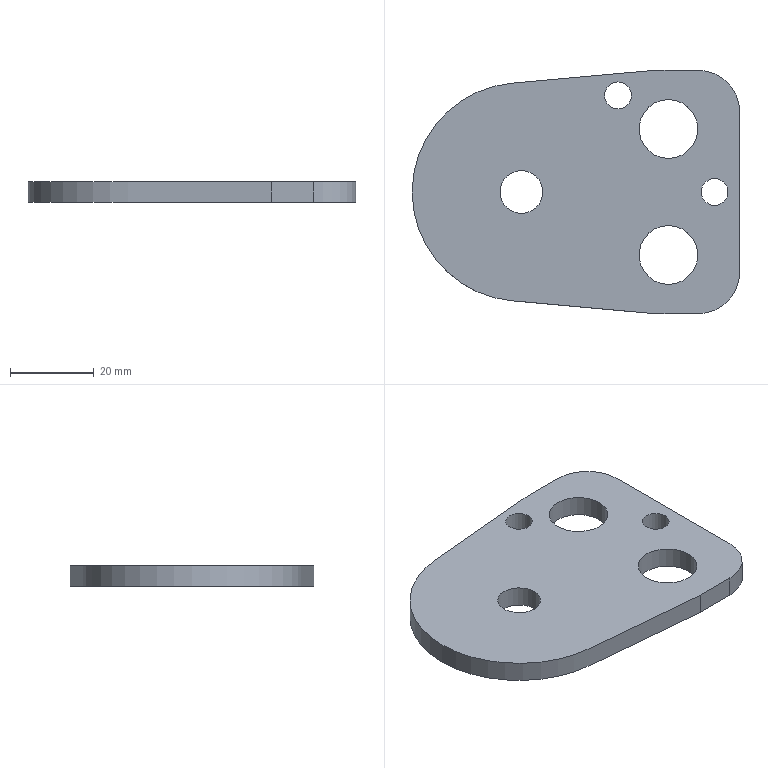Part | NX | features solid 2 | 1 solid | 17 faces | box 78 x 58 x 5 mm | volume 17443 mm3 | plane 9 | cylinder 8 | commonest cylinder face diameters 6.4 x2 14 x2 20 x2 10.2 x1 52 x1
STEP:
#1=CARTESIAN_POINT('',(-809.43,-240.038,136.));
#2=VERTEX_POINT('',#1);
#3=CARTESIAN_POINT('',(-809.43,-240.038,131.));
#4=VERTEX_POINT('',#3);
#5=CARTESIAN_POINT('',(-809.43,-240.038,131.));
#6=DIRECTION('',(0.,0.,-1.));
#7=VECTOR('',#6,1000.);
#8=LINE('',#5,#7);
#9=EDGE_CURVE('',#2,#4,#8,.T.);
#10=ORIENTED_EDGE('',*,*,#9,.F.);
#11=CARTESIAN_POINT('',(-809.43,-240.038,136.));
#12=VERTEX_POINT('',#11);
#13=CARTESIAN_POINT('',(-809.43,-214.144,136.));
#14=DIRECTION('',(0.,1.,0.));
#15=VECTOR('',#14,1000.);
#16=LINE('',#13,#15);
#17=EDGE_CURVE('',#2,#12,#16,.T.);
#18=ORIENTED_EDGE('',*,*,#17,.T.);
#19=CARTESIAN_POINT('',(-809.43,-240.038,131.));
#20=VERTEX_POINT('',#19);
#21=CARTESIAN_POINT('',(-809.43,-240.038,131.));
#22=DIRECTION('',(0.,0.,1.));
#23=VECTOR('',#22,1000.);
#24=LINE('',#21,#23);
#25=EDGE_CURVE('',#20,#12,#24,.T.);
#26=ORIENTED_EDGE('',*,*,#25,.F.);
#27=CARTESIAN_POINT('',(-809.43,-214.144,131.));
#28=DIRECTION('',(0.,-1.,0.));
#29=VECTOR('',#28,1000.);
#30=LINE('',#27,#29);
#31=EDGE_CURVE('',#20,#4,#30,.T.);
#32=ORIENTED_EDGE('',*,*,#31,.T.);
#33=EDGE_LOOP('',(#10,#18,#26,#32));
#34=FACE_BOUND('',#33,.T.);
#35=CARTESIAN_POINT('',(-809.43,-214.144,131.));
#36=DIRECTION('',(-1.,0.,0.));
#37=DIRECTION('',(0.,0.,1.));
#38=AXIS2_PLACEMENT_3D('',#35,#36,#37);
#39=PLANE('',#38);
#40=ADVANCED_FACE('',(#34),#39,.T.);
#41=CARTESIAN_POINT('',(-775.09,-185.144,136.));
#42=VERTEX_POINT('',#41);
#43=CARTESIAN_POINT('',(-809.43,-188.249,136.));
#44=VERTEX_POINT('',#43);
#45=CARTESIAN_POINT('',(-795.009,-186.945,136.));
#46=DIRECTION('',(-0.9959,-0.09007,0.));
#47=VECTOR('',#46,1000.);
#48=LINE('',#45,#47);
#49=EDGE_CURVE('',#42,#44,#48,.T.);
#50=ORIENTED_EDGE('',*,*,#49,.T.);
#51=CARTESIAN_POINT('',(-809.43,-188.249,136.));
#52=VERTEX_POINT('',#51);
#53=CARTESIAN_POINT('',(-809.43,-214.144,136.));
#54=DIRECTION('',(0.,1.,0.));
#55=VECTOR('',#54,1000.);
#56=LINE('',#53,#55);
#57=EDGE_CURVE('',#52,#44,#56,.T.);
#58=ORIENTED_EDGE('',*,*,#57,.F.);
#59=CARTESIAN_POINT('',(-807.09,-214.144,136.));
#60=DIRECTION('',(0.,0.,-1.));
#61=DIRECTION('',(0.,-1.,0.));
#62=AXIS2_PLACEMENT_3D('',#59,#60,#61);
#63=CIRCLE('',#62,26.);
#64=EDGE_CURVE('',#12,#52,#63,.T.);
#65=ORIENTED_EDGE('',*,*,#64,.F.);
#66=ORIENTED_EDGE('',*,*,#17,.F.);
#67=CARTESIAN_POINT('',(-775.09,-243.144,136.));
#68=VERTEX_POINT('',#67);
#69=CARTESIAN_POINT('',(-795.009,-241.342,136.));
#70=DIRECTION('',(0.9959,-0.09007,0.));
#71=VECTOR('',#70,1000.);
#72=LINE('',#69,#71);
#73=EDGE_CURVE('',#2,#68,#72,.T.);
#74=ORIENTED_EDGE('',*,*,#73,.T.);
#75=CARTESIAN_POINT('',(-765.09,-243.144,136.));
#76=VERTEX_POINT('',#75);
#77=CARTESIAN_POINT('',(-792.26,-243.144,136.));
#78=DIRECTION('',(-1.,0.,0.));
#79=VECTOR('',#78,1000.);
#80=LINE('',#77,#79);
#81=EDGE_CURVE('',#76,#68,#80,.T.);
#82=ORIENTED_EDGE('',*,*,#81,.F.);
#83=CARTESIAN_POINT('',(-755.09,-233.144,136.));
#84=VERTEX_POINT('',#83);
#85=CARTESIAN_POINT('',(-765.09,-233.144,136.));
#86=DIRECTION('',(0.,0.,1.));
#87=DIRECTION('',(0.,1.,0.));
#88=AXIS2_PLACEMENT_3D('',#85,#86,#87);
#89=CIRCLE('',#88,10.);
#90=EDGE_CURVE('',#76,#84,#89,.T.);
#91=ORIENTED_EDGE('',*,*,#90,.T.);
#92=CARTESIAN_POINT('',(-755.09,-195.144,136.));
#93=VERTEX_POINT('',#92);
#94=CARTESIAN_POINT('',(-755.09,-214.144,136.));
#95=DIRECTION('',(0.,-1.,0.));
#96=VECTOR('',#95,1000.);
#97=LINE('',#94,#96);
#98=EDGE_CURVE('',#93,#84,#97,.T.);
#99=ORIENTED_EDGE('',*,*,#98,.F.);
#100=CARTESIAN_POINT('',(-765.09,-185.144,136.));
#101=VERTEX_POINT('',#100);
#102=CARTESIAN_POINT('',(-765.09,-195.144,136.));
#103=DIRECTION('',(0.,0.,1.));
#104=DIRECTION('',(0.,1.,0.));
#105=AXIS2_PLACEMENT_3D('',#102,#103,#104);
#106=CIRCLE('',#105,10.);
#107=EDGE_CURVE('',#93,#101,#106,.T.);
#108=ORIENTED_EDGE('',*,*,#107,.T.);
#109=CARTESIAN_POINT('',(-792.26,-185.144,136.));
#110=DIRECTION('',(1.,0.,0.));
#111=VECTOR('',#110,1000.);
#112=LINE('',#109,#111);
#113=EDGE_CURVE('',#42,#101,#112,.T.);
#114=ORIENTED_EDGE('',*,*,#113,.F.);
#115=EDGE_LOOP('',(#50,#58,#65,#66,#74,#82,#91,#99,#108,#114));
#116=FACE_BOUND('',#115,.T.);
#117=CARTESIAN_POINT('',(-761.09,-217.344,136.));
#118=VERTEX_POINT('',#117);
#119=CARTESIAN_POINT('',(-761.09,-214.144,136.));
#120=DIRECTION('',(0.,0.,-1.));
#121=DIRECTION('',(0.,-1.,0.));
#122=AXIS2_PLACEMENT_3D('',#119,#120,#121);
#123=CIRCLE('',#122,3.2);
#124=EDGE_CURVE('',#118,#118,#123,.T.);
#125=ORIENTED_EDGE('',*,*,#124,.T.);
#126=EDGE_LOOP('',(#125));
#127=FACE_BOUND('',#126,.T.);
#128=CARTESIAN_POINT('',(-784.09,-194.344,136.));
#129=VERTEX_POINT('',#128);
#130=CARTESIAN_POINT('',(-784.09,-191.144,136.));
#131=DIRECTION('',(0.,0.,-1.));
#132=DIRECTION('',(0.,-1.,0.));
#133=AXIS2_PLACEMENT_3D('',#130,#131,#132);
#134=CIRCLE('',#133,3.2);
#135=EDGE_CURVE('',#129,#129,#134,.T.);
#136=ORIENTED_EDGE('',*,*,#135,.T.);
#137=EDGE_LOOP('',(#136));
#138=FACE_BOUND('',#137,.T.);
#139=CARTESIAN_POINT('',(-772.09,-206.144,136.));
#140=VERTEX_POINT('',#139);
#141=CARTESIAN_POINT('',(-772.09,-199.144,136.));
#142=DIRECTION('',(0.,0.,-1.));
#143=DIRECTION('',(0.,-1.,0.));
#144=AXIS2_PLACEMENT_3D('',#141,#142,#143);
#145=CIRCLE('',#144,7.);
#146=EDGE_CURVE('',#140,#140,#145,.T.);
#147=ORIENTED_EDGE('',*,*,#146,.T.);
#148=EDGE_LOOP('',(#147));
#149=FACE_BOUND('',#148,.T.);
#150=CARTESIAN_POINT('',(-772.09,-236.144,136.));
#151=VERTEX_POINT('',#150);
#152=CARTESIAN_POINT('',(-772.09,-229.144,136.));
#153=DIRECTION('',(0.,0.,-1.));
#154=DIRECTION('',(0.,-1.,0.));
#155=AXIS2_PLACEMENT_3D('',#152,#153,#154);
#156=CIRCLE('',#155,7.);
#157=EDGE_CURVE('',#151,#151,#156,.T.);
#158=ORIENTED_EDGE('',*,*,#157,.T.);
#159=EDGE_LOOP('',(#158));
#160=FACE_BOUND('',#159,.T.);
#161=CARTESIAN_POINT('',(-807.09,-219.244,136.));
#162=VERTEX_POINT('',#161);
#163=CARTESIAN_POINT('',(-807.09,-214.144,136.));
#164=DIRECTION('',(0.,0.,-1.));
#165=DIRECTION('',(0.,-1.,0.));
#166=AXIS2_PLACEMENT_3D('',#163,#164,#165);
#167=CIRCLE('',#166,5.1);
#168=EDGE_CURVE('',#162,#162,#167,.T.);
#169=ORIENTED_EDGE('',*,*,#168,.T.);
#170=EDGE_LOOP('',(#169));
#171=FACE_BOUND('',#170,.T.);
#172=CARTESIAN_POINT('',(-792.26,-214.144,136.));
#173=DIRECTION('',(0.,0.,1.));
#174=DIRECTION('',(0.,1.,0.));
#175=AXIS2_PLACEMENT_3D('',#172,#173,#174);
#176=PLANE('',#175);
#177=ADVANCED_FACE('',(#116,#127,#138,#149,#160,#171),#176,.T.);
#178=CARTESIAN_POINT('',(-775.09,-243.144,131.));
#179=VERTEX_POINT('',#178);
#180=CARTESIAN_POINT('',(-775.09,-243.144,131.));
#181=DIRECTION('',(0.,0.,1.));
#182=VECTOR('',#181,1000.);
#183=LINE('',#180,#182);
#184=EDGE_CURVE('',#179,#68,#183,.T.);
#185=ORIENTED_EDGE('',*,*,#184,.F.);
#186=CARTESIAN_POINT('',(-765.09,-243.144,131.));
#187=VERTEX_POINT('',#186);
#188=CARTESIAN_POINT('',(-792.26,-243.144,131.));
#189=DIRECTION('',(1.,0.,0.));
#190=VECTOR('',#189,1000.);
#191=LINE('',#188,#190);
#192=EDGE_CURVE('',#179,#187,#191,.T.);
#193=ORIENTED_EDGE('',*,*,#192,.T.);
#194=CARTESIAN_POINT('',(-765.09,-243.144,131.));
#195=DIRECTION('',(0.,0.,1.));
#196=VECTOR('',#195,1000.);
#197=LINE('',#194,#196);
#198=EDGE_CURVE('',#187,#76,#197,.T.);
#199=ORIENTED_EDGE('',*,*,#198,.T.);
#200=ORIENTED_EDGE('',*,*,#81,.T.);
#201=EDGE_LOOP('',(#185,#193,#199,#200));
#202=FACE_BOUND('',#201,.T.);
#203=CARTESIAN_POINT('',(-792.26,-243.144,131.));
#204=DIRECTION('',(0.,-1.,0.));
#205=DIRECTION('',(0.,0.,1.));
#206=AXIS2_PLACEMENT_3D('',#203,#204,#205);
#207=PLANE('',#206);
#208=ADVANCED_FACE('',(#202),#207,.T.);
#209=CARTESIAN_POINT('',(-809.43,-188.249,131.));
#210=VERTEX_POINT('',#209);
#211=CARTESIAN_POINT('',(-809.43,-188.249,131.));
#212=DIRECTION('',(0.,0.,1.));
#213=VECTOR('',#212,1000.);
#214=LINE('',#211,#213);
#215=EDGE_CURVE('',#210,#44,#214,.T.);
#216=ORIENTED_EDGE('',*,*,#215,.F.);
#217=CARTESIAN_POINT('',(-809.43,-188.249,131.));
#218=VERTEX_POINT('',#217);
#219=CARTESIAN_POINT('',(-809.43,-214.144,131.));
#220=DIRECTION('',(0.,-1.,0.));
#221=VECTOR('',#220,1000.);
#222=LINE('',#219,#221);
#223=EDGE_CURVE('',#210,#218,#222,.T.);
#224=ORIENTED_EDGE('',*,*,#223,.T.);
#225=CARTESIAN_POINT('',(-809.43,-188.249,131.));
#226=DIRECTION('',(0.,0.,1.));
#227=VECTOR('',#226,1000.);
#228=LINE('',#225,#227);
#229=EDGE_CURVE('',#52,#218,#228,.F.);
#230=ORIENTED_EDGE('',*,*,#229,.F.);
#231=ORIENTED_EDGE('',*,*,#57,.T.);
#232=EDGE_LOOP('',(#216,#224,#230,#231));
#233=FACE_BOUND('',#232,.T.);
#234=CARTESIAN_POINT('',(-809.43,-214.144,131.));
#235=DIRECTION('',(-1.,0.,0.));
#236=DIRECTION('',(0.,0.,1.));
#237=AXIS2_PLACEMENT_3D('',#234,#235,#236);
#238=PLANE('',#237);
#239=ADVANCED_FACE('',(#233),#238,.T.);
#240=CARTESIAN_POINT('',(-775.09,-185.144,131.));
#241=VERTEX_POINT('',#240);
#242=CARTESIAN_POINT('',(-795.009,-186.945,131.));
#243=DIRECTION('',(0.9959,0.09007,0.));
#244=VECTOR('',#243,1000.);
#245=LINE('',#242,#244);
#246=EDGE_CURVE('',#210,#241,#245,.T.);
#247=ORIENTED_EDGE('',*,*,#246,.T.);
#248=CARTESIAN_POINT('',(-765.09,-185.144,131.));
#249=VERTEX_POINT('',#248);
#250=CARTESIAN_POINT('',(-792.26,-185.144,131.));
#251=DIRECTION('',(-1.,0.,0.));
#252=VECTOR('',#251,1000.);
#253=LINE('',#250,#252);
#254=EDGE_CURVE('',#249,#241,#253,.T.);
#255=ORIENTED_EDGE('',*,*,#254,.F.);
#256=CARTESIAN_POINT('',(-755.09,-195.144,131.));
#257=VERTEX_POINT('',#256);
#258=CARTESIAN_POINT('',(-765.09,-195.144,131.));
#259=DIRECTION('',(0.,0.,-1.));
#260=DIRECTION('',(0.,-1.,0.));
#261=AXIS2_PLACEMENT_3D('',#258,#259,#260);
#262=CIRCLE('',#261,10.);
#263=EDGE_CURVE('',#249,#257,#262,.T.);
#264=ORIENTED_EDGE('',*,*,#263,.T.);
#265=CARTESIAN_POINT('',(-755.09,-233.144,131.));
#266=VERTEX_POINT('',#265);
#267=CARTESIAN_POINT('',(-755.09,-214.144,131.));
#268=DIRECTION('',(0.,1.,0.));
#269=VECTOR('',#268,1000.);
#270=LINE('',#267,#269);
#271=EDGE_CURVE('',#266,#257,#270,.T.);
#272=ORIENTED_EDGE('',*,*,#271,.F.);
#273=CARTESIAN_POINT('',(-765.09,-233.144,131.));
#274=DIRECTION('',(0.,0.,-1.));
#275=DIRECTION('',(0.,-1.,0.));
#276=AXIS2_PLACEMENT_3D('',#273,#274,#275);
#277=CIRCLE('',#276,10.);
#278=EDGE_CURVE('',#266,#187,#277,.T.);
#279=ORIENTED_EDGE('',*,*,#278,.T.);
#280=ORIENTED_EDGE('',*,*,#192,.F.);
#281=CARTESIAN_POINT('',(-795.009,-241.342,131.));
#282=DIRECTION('',(-0.9959,0.09007,0.));
#283=VECTOR('',#282,1000.);
#284=LINE('',#281,#283);
#285=EDGE_CURVE('',#179,#4,#284,.T.);
#286=ORIENTED_EDGE('',*,*,#285,.T.);
#287=ORIENTED_EDGE('',*,*,#31,.F.);
#288=CARTESIAN_POINT('',(-807.09,-214.144,131.));
#289=DIRECTION('',(0.,0.,1.));
#290=DIRECTION('',(0.,1.,0.));
#291=AXIS2_PLACEMENT_3D('',#288,#289,#290);
#292=CIRCLE('',#291,26.);
#293=EDGE_CURVE('',#218,#20,#292,.T.);
#294=ORIENTED_EDGE('',*,*,#293,.F.);
#295=ORIENTED_EDGE('',*,*,#223,.F.);
#296=EDGE_LOOP('',(#247,#255,#264,#272,#279,#280,#286,#287,#294,#295));
#297=FACE_BOUND('',#296,.T.);
#298=CARTESIAN_POINT('',(-761.09,-210.944,131.));
#299=VERTEX_POINT('',#298);
#300=CARTESIAN_POINT('',(-761.09,-214.144,131.));
#301=DIRECTION('',(0.,0.,1.));
#302=DIRECTION('',(0.,1.,0.));
#303=AXIS2_PLACEMENT_3D('',#300,#301,#302);
#304=CIRCLE('',#303,3.2);
#305=EDGE_CURVE('',#299,#299,#304,.T.);
#306=ORIENTED_EDGE('',*,*,#305,.T.);
#307=EDGE_LOOP('',(#306));
#308=FACE_BOUND('',#307,.T.);
#309=CARTESIAN_POINT('',(-784.09,-187.944,131.));
#310=VERTEX_POINT('',#309);
#311=CARTESIAN_POINT('',(-784.09,-191.144,131.));
#312=DIRECTION('',(0.,0.,1.));
#313=DIRECTION('',(0.,1.,0.));
#314=AXIS2_PLACEMENT_3D('',#311,#312,#313);
#315=CIRCLE('',#314,3.2);
#316=EDGE_CURVE('',#310,#310,#315,.T.);
#317=ORIENTED_EDGE('',*,*,#316,.T.);
#318=EDGE_LOOP('',(#317));
#319=FACE_BOUND('',#318,.T.);
#320=CARTESIAN_POINT('',(-772.09,-192.144,131.));
#321=VERTEX_POINT('',#320);
#322=CARTESIAN_POINT('',(-772.09,-199.144,131.));
#323=DIRECTION('',(0.,0.,1.));
#324=DIRECTION('',(0.,1.,0.));
#325=AXIS2_PLACEMENT_3D('',#322,#323,#324);
#326=CIRCLE('',#325,7.);
#327=EDGE_CURVE('',#321,#321,#326,.T.);
#328=ORIENTED_EDGE('',*,*,#327,.T.);
#329=EDGE_LOOP('',(#328));
#330=FACE_BOUND('',#329,.T.);
#331=CARTESIAN_POINT('',(-772.09,-222.144,131.));
#332=VERTEX_POINT('',#331);
#333=CARTESIAN_POINT('',(-772.09,-229.144,131.));
#334=DIRECTION('',(0.,0.,1.));
#335=DIRECTION('',(0.,1.,0.));
#336=AXIS2_PLACEMENT_3D('',#333,#334,#335);
#337=CIRCLE('',#336,7.);
#338=EDGE_CURVE('',#332,#332,#337,.T.);
#339=ORIENTED_EDGE('',*,*,#338,.T.);
#340=EDGE_LOOP('',(#339));
#341=FACE_BOUND('',#340,.T.);
#342=CARTESIAN_POINT('',(-807.09,-209.044,131.));
#343=VERTEX_POINT('',#342);
#344=CARTESIAN_POINT('',(-807.09,-214.144,131.));
#345=DIRECTION('',(0.,0.,1.));
#346=DIRECTION('',(0.,1.,0.));
#347=AXIS2_PLACEMENT_3D('',#344,#345,#346);
#348=CIRCLE('',#347,5.1);
#349=EDGE_CURVE('',#343,#343,#348,.T.);
#350=ORIENTED_EDGE('',*,*,#349,.T.);
#351=EDGE_LOOP('',(#350));
#352=FACE_BOUND('',#351,.T.);
#353=CARTESIAN_POINT('',(-792.26,-214.144,131.));
#354=DIRECTION('',(0.,0.,-1.));
#355=DIRECTION('',(0.,-1.,0.));
#356=AXIS2_PLACEMENT_3D('',#353,#354,#355);
#357=PLANE('',#356);
#358=ADVANCED_FACE('',(#297,#308,#319,#330,#341,#352),#357,.T.);
#359=CARTESIAN_POINT('',(-775.09,-185.144,131.));
#360=DIRECTION('',(0.,0.,1.));
#361=VECTOR('',#360,1000.);
#362=LINE('',#359,#361);
#363=EDGE_CURVE('',#241,#42,#362,.T.);
#364=ORIENTED_EDGE('',*,*,#363,.T.);
#365=ORIENTED_EDGE('',*,*,#113,.T.);
#366=CARTESIAN_POINT('',(-765.09,-185.144,131.));
#367=DIRECTION('',(0.,0.,1.));
#368=VECTOR('',#367,1000.);
#369=LINE('',#366,#368);
#370=EDGE_CURVE('',#101,#249,#369,.F.);
#371=ORIENTED_EDGE('',*,*,#370,.T.);
#372=ORIENTED_EDGE('',*,*,#254,.T.);
#373=EDGE_LOOP('',(#364,#365,#371,#372));
#374=FACE_BOUND('',#373,.T.);
#375=CARTESIAN_POINT('',(-792.26,-185.144,131.));
#376=DIRECTION('',(0.,1.,0.));
#377=DIRECTION('',(0.,0.,-1.));
#378=AXIS2_PLACEMENT_3D('',#375,#376,#377);
#379=PLANE('',#378);
#380=ADVANCED_FACE('',(#374),#379,.T.);
#381=ORIENTED_EDGE('',*,*,#293,.T.);
#382=ORIENTED_EDGE('',*,*,#25,.T.);
#383=ORIENTED_EDGE('',*,*,#64,.T.);
#384=ORIENTED_EDGE('',*,*,#229,.T.);
#385=EDGE_LOOP('',(#381,#382,#383,#384));
#386=FACE_BOUND('',#385,.T.);
#387=CARTESIAN_POINT('',(-807.09,-214.144,131.));
#388=DIRECTION('',(0.,0.,1.));
#389=DIRECTION('',(0.,1.,0.));
#390=AXIS2_PLACEMENT_3D('',#387,#388,#389);
#391=CYLINDRICAL_SURFACE('',#390,26.);
#392=ADVANCED_FACE('',(#386),#391,.T.);
#393=ORIENTED_EDGE('',*,*,#271,.T.);
#394=CARTESIAN_POINT('',(-755.09,-195.144,131.));
#395=DIRECTION('',(0.,0.,1.));
#396=VECTOR('',#395,1000.);
#397=LINE('',#394,#396);
#398=EDGE_CURVE('',#257,#93,#397,.T.);
#399=ORIENTED_EDGE('',*,*,#398,.T.);
#400=ORIENTED_EDGE('',*,*,#98,.T.);
#401=CARTESIAN_POINT('',(-755.09,-233.144,131.));
#402=DIRECTION('',(0.,0.,1.));
#403=VECTOR('',#402,1000.);
#404=LINE('',#401,#403);
#405=EDGE_CURVE('',#84,#266,#404,.F.);
#406=ORIENTED_EDGE('',*,*,#405,.T.);
#407=EDGE_LOOP('',(#393,#399,#400,#406));
#408=FACE_BOUND('',#407,.T.);
#409=CARTESIAN_POINT('',(-755.09,-214.144,131.));
#410=DIRECTION('',(1.,0.,0.));
#411=DIRECTION('',(0.,0.,-1.));
#412=AXIS2_PLACEMENT_3D('',#409,#410,#411);
#413=PLANE('',#412);
#414=ADVANCED_FACE('',(#408),#413,.T.);
#415=ORIENTED_EDGE('',*,*,#168,.F.);
#416=EDGE_LOOP('',(#415));
#417=FACE_BOUND('',#416,.T.);
#418=ORIENTED_EDGE('',*,*,#349,.F.);
#419=EDGE_LOOP('',(#418));
#420=FACE_BOUND('',#419,.T.);
#421=CARTESIAN_POINT('',(-807.09,-214.144,131.));
#422=DIRECTION('',(0.,0.,1.));
#423=DIRECTION('',(0.,1.,0.));
#424=AXIS2_PLACEMENT_3D('',#421,#422,#423);
#425=CYLINDRICAL_SURFACE('',#424,5.1);
#426=ADVANCED_FACE('',(#417,#420),#425,.F.);
#427=ORIENTED_EDGE('',*,*,#157,.F.);
#428=EDGE_LOOP('',(#427));
#429=FACE_BOUND('',#428,.T.);
#430=ORIENTED_EDGE('',*,*,#338,.F.);
#431=EDGE_LOOP('',(#430));
#432=FACE_BOUND('',#431,.T.);
#433=CARTESIAN_POINT('',(-772.09,-229.144,131.));
#434=DIRECTION('',(0.,0.,1.));
#435=DIRECTION('',(0.,1.,0.));
#436=AXIS2_PLACEMENT_3D('',#433,#434,#435);
#437=CYLINDRICAL_SURFACE('',#436,7.);
#438=ADVANCED_FACE('',(#429,#432),#437,.F.);
#439=ORIENTED_EDGE('',*,*,#146,.F.);
#440=EDGE_LOOP('',(#439));
#441=FACE_BOUND('',#440,.T.);
#442=ORIENTED_EDGE('',*,*,#327,.F.);
#443=EDGE_LOOP('',(#442));
#444=FACE_BOUND('',#443,.T.);
#445=CARTESIAN_POINT('',(-772.09,-199.144,131.));
#446=DIRECTION('',(0.,0.,1.));
#447=DIRECTION('',(0.,1.,0.));
#448=AXIS2_PLACEMENT_3D('',#445,#446,#447);
#449=CYLINDRICAL_SURFACE('',#448,7.);
#450=ADVANCED_FACE('',(#441,#444),#449,.F.);
#451=ORIENTED_EDGE('',*,*,#135,.F.);
#452=EDGE_LOOP('',(#451));
#453=FACE_BOUND('',#452,.T.);
#454=ORIENTED_EDGE('',*,*,#316,.F.);
#455=EDGE_LOOP('',(#454));
#456=FACE_BOUND('',#455,.T.);
#457=CARTESIAN_POINT('',(-784.09,-191.144,131.));
#458=DIRECTION('',(0.,0.,1.));
#459=DIRECTION('',(0.,1.,0.));
#460=AXIS2_PLACEMENT_3D('',#457,#458,#459);
#461=CYLINDRICAL_SURFACE('',#460,3.2);
#462=ADVANCED_FACE('',(#453,#456),#461,.F.);
#463=ORIENTED_EDGE('',*,*,#124,.F.);
#464=EDGE_LOOP('',(#463));
#465=FACE_BOUND('',#464,.T.);
#466=ORIENTED_EDGE('',*,*,#305,.F.);
#467=EDGE_LOOP('',(#466));
#468=FACE_BOUND('',#467,.T.);
#469=CARTESIAN_POINT('',(-761.09,-214.144,131.));
#470=DIRECTION('',(0.,0.,1.));
#471=DIRECTION('',(0.,1.,0.));
#472=AXIS2_PLACEMENT_3D('',#469,#470,#471);
#473=CYLINDRICAL_SURFACE('',#472,3.2);
#474=ADVANCED_FACE('',(#465,#468),#473,.F.);
#475=ORIENTED_EDGE('',*,*,#263,.F.);
#476=ORIENTED_EDGE('',*,*,#370,.F.);
#477=ORIENTED_EDGE('',*,*,#107,.F.);
#478=ORIENTED_EDGE('',*,*,#398,.F.);
#479=EDGE_LOOP('',(#475,#476,#477,#478));
#480=FACE_BOUND('',#479,.T.);
#481=CARTESIAN_POINT('',(-765.09,-195.144,131.));
#482=DIRECTION('',(0.,0.,1.));
#483=DIRECTION('',(0.,1.,0.));
#484=AXIS2_PLACEMENT_3D('',#481,#482,#483);
#485=CYLINDRICAL_SURFACE('',#484,10.);
#486=ADVANCED_FACE('',(#480),#485,.T.);
#487=ORIENTED_EDGE('',*,*,#278,.F.);
#488=ORIENTED_EDGE('',*,*,#405,.F.);
#489=ORIENTED_EDGE('',*,*,#90,.F.);
#490=ORIENTED_EDGE('',*,*,#198,.F.);
#491=EDGE_LOOP('',(#487,#488,#489,#490));
#492=FACE_BOUND('',#491,.T.);
#493=CARTESIAN_POINT('',(-765.09,-233.144,131.));
#494=DIRECTION('',(0.,0.,1.));
#495=DIRECTION('',(0.,1.,0.));
#496=AXIS2_PLACEMENT_3D('',#493,#494,#495);
#497=CYLINDRICAL_SURFACE('',#496,10.);
#498=ADVANCED_FACE('',(#492),#497,.T.);
#499=ORIENTED_EDGE('',*,*,#9,.T.);
#500=ORIENTED_EDGE('',*,*,#285,.F.);
#501=ORIENTED_EDGE('',*,*,#184,.T.);
#502=ORIENTED_EDGE('',*,*,#73,.F.);
#503=EDGE_LOOP('',(#499,#500,#501,#502));
#504=FACE_BOUND('',#503,.T.);
#505=CARTESIAN_POINT('',(-795.009,-241.342,131.));
#506=DIRECTION('',(0.09007,0.9959,0.));
#507=DIRECTION('',(0.,0.,-1.));
#508=AXIS2_PLACEMENT_3D('',#505,#506,#507);
#509=PLANE('',#508);
#510=ADVANCED_FACE('',(#504),#509,.F.);
#511=ORIENTED_EDGE('',*,*,#215,.T.);
#512=ORIENTED_EDGE('',*,*,#49,.F.);
#513=ORIENTED_EDGE('',*,*,#363,.F.);
#514=ORIENTED_EDGE('',*,*,#246,.F.);
#515=EDGE_LOOP('',(#511,#512,#513,#514));
#516=FACE_BOUND('',#515,.T.);
#517=CARTESIAN_POINT('',(-795.009,-186.945,131.));
#518=DIRECTION('',(0.09007,-0.9959,0.));
#519=DIRECTION('',(0.,0.,1.));
#520=AXIS2_PLACEMENT_3D('',#517,#518,#519);
#521=PLANE('',#520);
#522=ADVANCED_FACE('',(#516),#521,.F.);
#523=CLOSED_SHELL('',(#40,#177,#208,#239,#358,#380,#392,#414,#426,#438,#450,#462,#474,#486,#498,#510,#522));
#524=MANIFOLD_SOLID_BREP('',#523);
#525=(LENGTH_UNIT()NAMED_UNIT(*)SI_UNIT(.MILLI.,.METRE.));
#526=UNCERTAINTY_MEASURE_WITH_UNIT(LENGTH_MEASURE(0.00001),#525,'','');
#527=(NAMED_UNIT(*)PLANE_ANGLE_UNIT()SI_UNIT($,.RADIAN.));
#528=(NAMED_UNIT(*)SI_UNIT($,.STERADIAN.)SOLID_ANGLE_UNIT());
#529=(GEOMETRIC_REPRESENTATION_CONTEXT(3)GLOBAL_UNCERTAINTY_ASSIGNED_CONTEXT((#526))GLOBAL_UNIT_ASSIGNED_CONTEXT((#525,#527,#528))REPRESENTATION_CONTEXT('',''));
#530=ADVANCED_BREP_SHAPE_REPRESENTATION('',(#524),#529);